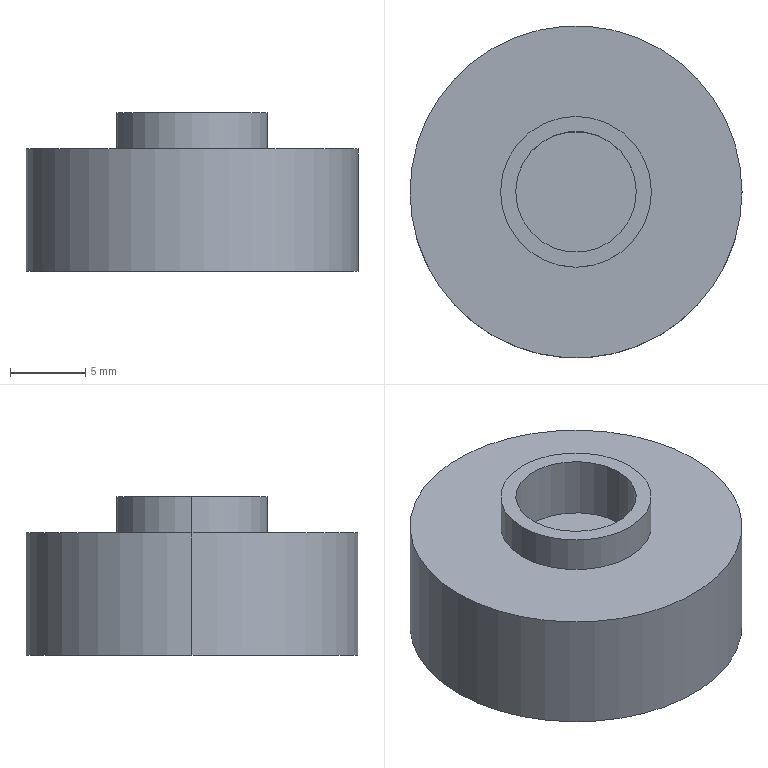Part | SolidWorks | features ICE 3, Chamfer 1, Extrusion 1 | 1 solid | 15 faces | box 22 x 22 x 10.5 mm | volume 2336 mm3 | cylinder 8 | plane 5 | cone 2 | commonest cylinder face diameters 8 x2 10 x2 17.5 x2 22 x2
STEP:
#1=CARTESIAN_POINT('',(8.75,0.,0.2));
#2=VERTEX_POINT('',#1);
#3=CARTESIAN_POINT('',(-8.75,0.,0.2));
#4=VERTEX_POINT('',#3);
#5=CARTESIAN_POINT('',(0.,0.,0.2));
#6=DIRECTION('',(0.,0.,-1.));
#7=DIRECTION('',(1.,0.,0.));
#8=AXIS2_PLACEMENT_3D('',#5,#6,#7);
#9=CIRCLE('',#8,8.75);
#10=EDGE_CURVE('',#2,#4,#9,.T.);
#11=ORIENTED_EDGE('',*,*,#10,.F.);
#12=CARTESIAN_POINT('',(8.95,0.,0.));
#13=VERTEX_POINT('',#12);
#14=CARTESIAN_POINT('',(8.75,0.,0.2));
#15=DIRECTION('',(0.7071,0.,-0.7071));
#16=VECTOR('',#15,1000.);
#17=LINE('',#14,#16);
#18=EDGE_CURVE('',#2,#13,#17,.T.);
#19=ORIENTED_EDGE('',*,*,#18,.T.);
#20=CARTESIAN_POINT('',(-8.95,0.,0.));
#21=VERTEX_POINT('',#20);
#22=CARTESIAN_POINT('',(0.,0.,0.));
#23=DIRECTION('',(0.,0.,1.));
#24=DIRECTION('',(1.,0.,0.));
#25=AXIS2_PLACEMENT_3D('',#22,#23,#24);
#26=CIRCLE('',#25,8.95);
#27=EDGE_CURVE('',#21,#13,#26,.T.);
#28=ORIENTED_EDGE('',*,*,#27,.F.);
#29=CARTESIAN_POINT('',(-8.75,0.,0.2));
#30=DIRECTION('',(-0.7071,0.,-0.7071));
#31=VECTOR('',#30,1000.);
#32=LINE('',#29,#31);
#33=EDGE_CURVE('',#4,#21,#32,.T.);
#34=ORIENTED_EDGE('',*,*,#33,.F.);
#35=EDGE_LOOP('',(#11,#19,#28,#34));
#36=FACE_OUTER_BOUND('',#35,.T.);
#37=CARTESIAN_POINT('',(0.,0.,0.2));
#38=DIRECTION('',(0.,0.,-1.));
#39=DIRECTION('',(-1.,0.,0.));
#40=AXIS2_PLACEMENT_3D('',#37,#38,#39);
#41=CONICAL_SURFACE('',#40,8.75,0.7854);
#42=ADVANCED_FACE('',(#36),#41,.F.);
#43=CARTESIAN_POINT('',(8.75,0.,3.));
#44=VERTEX_POINT('',#43);
#45=CARTESIAN_POINT('',(-8.75,0.,3.));
#46=VERTEX_POINT('',#45);
#47=CARTESIAN_POINT('',(0.,0.,3.));
#48=DIRECTION('',(0.,0.,-1.));
#49=DIRECTION('',(-1.,0.,0.));
#50=AXIS2_PLACEMENT_3D('',#47,#48,#49);
#51=CIRCLE('',#50,8.75);
#52=EDGE_CURVE('',#44,#46,#51,.T.);
#53=ORIENTED_EDGE('',*,*,#52,.F.);
#54=CARTESIAN_POINT('',(8.75,0.,3.));
#55=DIRECTION('',(0.,0.,-1.));
#56=VECTOR('',#55,1000.);
#57=LINE('',#54,#56);
#58=EDGE_CURVE('',#44,#2,#57,.T.);
#59=ORIENTED_EDGE('',*,*,#58,.T.);
#60=ORIENTED_EDGE('',*,*,#10,.T.);
#61=CARTESIAN_POINT('',(-8.75,0.,3.));
#62=DIRECTION('',(0.,0.,-1.));
#63=VECTOR('',#62,1000.);
#64=LINE('',#61,#63);
#65=EDGE_CURVE('',#46,#4,#64,.T.);
#66=ORIENTED_EDGE('',*,*,#65,.F.);
#67=EDGE_LOOP('',(#53,#59,#60,#66));
#68=FACE_OUTER_BOUND('',#67,.T.);
#69=CARTESIAN_POINT('',(0.,0.,3.));
#70=DIRECTION('',(0.,0.,-1.));
#71=DIRECTION('',(-1.,0.,0.));
#72=AXIS2_PLACEMENT_3D('',#69,#70,#71);
#73=CYLINDRICAL_SURFACE('',#72,8.75);
#74=ADVANCED_FACE('',(#68),#73,.F.);
#75=CARTESIAN_POINT('',(-4.,0.,6.35));
#76=VERTEX_POINT('',#75);
#77=CARTESIAN_POINT('',(4.,0.,6.35));
#78=VERTEX_POINT('',#77);
#79=CARTESIAN_POINT('',(0.,0.,6.35));
#80=DIRECTION('',(0.,0.,1.));
#81=DIRECTION('',(1.,0.,0.));
#82=AXIS2_PLACEMENT_3D('',#79,#80,#81);
#83=CIRCLE('',#82,4.);
#84=EDGE_CURVE('',#76,#78,#83,.T.);
#85=ORIENTED_EDGE('',*,*,#84,.F.);
#86=CARTESIAN_POINT('',(-4.,0.,10.5));
#87=VERTEX_POINT('',#86);
#88=CARTESIAN_POINT('',(-4.,0.,6.35));
#89=DIRECTION('',(0.,0.,1.));
#90=VECTOR('',#89,1000.);
#91=LINE('',#88,#90);
#92=EDGE_CURVE('',#76,#87,#91,.T.);
#93=ORIENTED_EDGE('',*,*,#92,.T.);
#94=CARTESIAN_POINT('',(4.,0.,10.5));
#95=VERTEX_POINT('',#94);
#96=CARTESIAN_POINT('',(0.,0.,10.5));
#97=DIRECTION('',(0.,0.,1.));
#98=DIRECTION('',(1.,0.,0.));
#99=AXIS2_PLACEMENT_3D('',#96,#97,#98);
#100=CIRCLE('',#99,4.);
#101=EDGE_CURVE('',#87,#95,#100,.T.);
#102=ORIENTED_EDGE('',*,*,#101,.T.);
#103=CARTESIAN_POINT('',(4.,0.,6.35));
#104=DIRECTION('',(0.,0.,1.));
#105=VECTOR('',#104,1000.);
#106=LINE('',#103,#105);
#107=EDGE_CURVE('',#78,#95,#106,.T.);
#108=ORIENTED_EDGE('',*,*,#107,.F.);
#109=EDGE_LOOP('',(#85,#93,#102,#108));
#110=FACE_OUTER_BOUND('',#109,.T.);
#111=CARTESIAN_POINT('',(0.,0.,6.35));
#112=DIRECTION('',(0.,0.,1.));
#113=DIRECTION('',(1.,0.,0.));
#114=AXIS2_PLACEMENT_3D('',#111,#112,#113);
#115=CYLINDRICAL_SURFACE('',#114,4.);
#116=ADVANCED_FACE('',(#110),#115,.F.);
#117=CARTESIAN_POINT('',(5.,0.,8.1));
#118=VERTEX_POINT('',#117);
#119=CARTESIAN_POINT('',(-5.,0.,8.1));
#120=VERTEX_POINT('',#119);
#121=CARTESIAN_POINT('',(0.,0.,8.1));
#122=DIRECTION('',(0.,0.,1.));
#123=DIRECTION('',(1.,0.,0.));
#124=AXIS2_PLACEMENT_3D('',#121,#122,#123);
#125=CIRCLE('',#124,5.);
#126=EDGE_CURVE('',#118,#120,#125,.T.);
#127=ORIENTED_EDGE('',*,*,#126,.T.);
#128=CARTESIAN_POINT('',(-5.,0.,10.5));
#129=VERTEX_POINT('',#128);
#130=CARTESIAN_POINT('',(-5.,0.,8.1));
#131=DIRECTION('',(0.,0.,1.));
#132=VECTOR('',#131,1000.);
#133=LINE('',#130,#132);
#134=EDGE_CURVE('',#120,#129,#133,.T.);
#135=ORIENTED_EDGE('',*,*,#134,.T.);
#136=CARTESIAN_POINT('',(5.,0.,10.5));
#137=VERTEX_POINT('',#136);
#138=CARTESIAN_POINT('',(0.,0.,10.5));
#139=DIRECTION('',(0.,0.,1.));
#140=DIRECTION('',(1.,0.,0.));
#141=AXIS2_PLACEMENT_3D('',#138,#139,#140);
#142=CIRCLE('',#141,5.);
#143=EDGE_CURVE('',#137,#129,#142,.T.);
#144=ORIENTED_EDGE('',*,*,#143,.F.);
#145=CARTESIAN_POINT('',(5.,0.,8.1));
#146=DIRECTION('',(0.,0.,1.));
#147=VECTOR('',#146,1000.);
#148=LINE('',#145,#147);
#149=EDGE_CURVE('',#118,#137,#148,.T.);
#150=ORIENTED_EDGE('',*,*,#149,.F.);
#151=EDGE_LOOP('',(#127,#135,#144,#150));
#152=FACE_OUTER_BOUND('',#151,.T.);
#153=CARTESIAN_POINT('',(0.,0.,8.1));
#154=DIRECTION('',(0.,0.,1.));
#155=DIRECTION('',(1.,0.,0.));
#156=AXIS2_PLACEMENT_3D('',#153,#154,#155);
#157=CYLINDRICAL_SURFACE('',#156,5.);
#158=ADVANCED_FACE('',(#152),#157,.T.);
#159=CARTESIAN_POINT('',(11.,0.,8.1));
#160=VERTEX_POINT('',#159);
#161=CARTESIAN_POINT('',(-11.,0.,8.1));
#162=VERTEX_POINT('',#161);
#163=CARTESIAN_POINT('',(0.,0.,8.1));
#164=DIRECTION('',(0.,0.,1.));
#165=DIRECTION('',(1.,0.,0.));
#166=AXIS2_PLACEMENT_3D('',#163,#164,#165);
#167=CIRCLE('',#166,11.);
#168=EDGE_CURVE('',#160,#162,#167,.T.);
#169=ORIENTED_EDGE('',*,*,#168,.F.);
#170=CARTESIAN_POINT('',(11.,0.,0.));
#171=VERTEX_POINT('',#170);
#172=CARTESIAN_POINT('',(11.,0.,10.5));
#173=DIRECTION('',(0.,0.,-1.));
#174=VECTOR('',#173,1000.);
#175=LINE('',#172,#174);
#176=EDGE_CURVE('',#160,#171,#175,.T.);
#177=ORIENTED_EDGE('',*,*,#176,.T.);
#178=CARTESIAN_POINT('',(-11.,0.,0.));
#179=VERTEX_POINT('',#178);
#180=CARTESIAN_POINT('',(0.,0.,0.));
#181=DIRECTION('',(0.,0.,1.));
#182=DIRECTION('',(1.,0.,0.));
#183=AXIS2_PLACEMENT_3D('',#180,#181,#182);
#184=CIRCLE('',#183,11.);
#185=EDGE_CURVE('',#171,#179,#184,.T.);
#186=ORIENTED_EDGE('',*,*,#185,.T.);
#187=CARTESIAN_POINT('',(-11.,0.,10.5));
#188=DIRECTION('',(0.,0.,-1.));
#189=VECTOR('',#188,1000.);
#190=LINE('',#187,#189);
#191=EDGE_CURVE('',#162,#179,#190,.T.);
#192=ORIENTED_EDGE('',*,*,#191,.F.);
#193=EDGE_LOOP('',(#169,#177,#186,#192));
#194=FACE_OUTER_BOUND('',#193,.T.);
#195=CARTESIAN_POINT('',(0.,0.,10.5));
#196=DIRECTION('',(0.,0.,-1.));
#197=DIRECTION('',(-1.,0.,0.));
#198=AXIS2_PLACEMENT_3D('',#195,#196,#197);
#199=CYLINDRICAL_SURFACE('',#198,11.);
#200=ADVANCED_FACE('',(#194),#199,.T.);
#201=ORIENTED_EDGE('',*,*,#176,.F.);
#202=CARTESIAN_POINT('',(0.,0.,8.1));
#203=DIRECTION('',(0.,0.,1.));
#204=DIRECTION('',(1.,0.,0.));
#205=AXIS2_PLACEMENT_3D('',#202,#203,#204);
#206=CIRCLE('',#205,11.);
#207=EDGE_CURVE('',#162,#160,#206,.T.);
#208=ORIENTED_EDGE('',*,*,#207,.F.);
#209=ORIENTED_EDGE('',*,*,#191,.T.);
#210=CARTESIAN_POINT('',(0.,0.,0.));
#211=DIRECTION('',(0.,0.,1.));
#212=DIRECTION('',(1.,0.,0.));
#213=AXIS2_PLACEMENT_3D('',#210,#211,#212);
#214=CIRCLE('',#213,11.);
#215=EDGE_CURVE('',#179,#171,#214,.T.);
#216=ORIENTED_EDGE('',*,*,#215,.T.);
#217=EDGE_LOOP('',(#201,#208,#209,#216));
#218=FACE_OUTER_BOUND('',#217,.T.);
#219=CARTESIAN_POINT('',(0.,0.,10.5));
#220=DIRECTION('',(0.,0.,-1.));
#221=DIRECTION('',(-1.,0.,0.));
#222=AXIS2_PLACEMENT_3D('',#219,#220,#221);
#223=CYLINDRICAL_SURFACE('',#222,11.);
#224=ADVANCED_FACE('',(#218),#223,.T.);
#225=ORIENTED_EDGE('',*,*,#27,.T.);
#226=CARTESIAN_POINT('',(0.,0.,0.));
#227=DIRECTION('',(0.,0.,1.));
#228=DIRECTION('',(1.,0.,0.));
#229=AXIS2_PLACEMENT_3D('',#226,#227,#228);
#230=CIRCLE('',#229,8.95);
#231=EDGE_CURVE('',#13,#21,#230,.T.);
#232=ORIENTED_EDGE('',*,*,#231,.T.);
#233=EDGE_LOOP('',(#225,#232));
#234=FACE_BOUND('',#233,.T.);
#235=ORIENTED_EDGE('',*,*,#215,.F.);
#236=ORIENTED_EDGE('',*,*,#185,.F.);
#237=EDGE_LOOP('',(#235,#236));
#238=FACE_OUTER_BOUND('',#237,.T.);
#239=CARTESIAN_POINT('',(0.,0.,0.));
#240=DIRECTION('',(0.,0.,1.));
#241=DIRECTION('',(1.,0.,0.));
#242=AXIS2_PLACEMENT_3D('',#239,#240,#241);
#243=PLANE('',#242);
#244=ADVANCED_FACE('',(#234,#238),#243,.F.);
#245=ORIENTED_EDGE('',*,*,#126,.F.);
#246=CARTESIAN_POINT('',(0.,0.,8.1));
#247=DIRECTION('',(0.,0.,1.));
#248=DIRECTION('',(1.,0.,0.));
#249=AXIS2_PLACEMENT_3D('',#246,#247,#248);
#250=CIRCLE('',#249,5.);
#251=EDGE_CURVE('',#120,#118,#250,.T.);
#252=ORIENTED_EDGE('',*,*,#251,.F.);
#253=EDGE_LOOP('',(#245,#252));
#254=FACE_BOUND('',#253,.T.);
#255=ORIENTED_EDGE('',*,*,#207,.T.);
#256=ORIENTED_EDGE('',*,*,#168,.T.);
#257=EDGE_LOOP('',(#255,#256));
#258=FACE_OUTER_BOUND('',#257,.T.);
#259=CARTESIAN_POINT('',(0.,0.,8.1));
#260=DIRECTION('',(0.,0.,1.));
#261=DIRECTION('',(1.,0.,0.));
#262=AXIS2_PLACEMENT_3D('',#259,#260,#261);
#263=PLANE('',#262);
#264=ADVANCED_FACE('',(#254,#258),#263,.T.);
#265=ORIENTED_EDGE('',*,*,#134,.F.);
#266=ORIENTED_EDGE('',*,*,#251,.T.);
#267=ORIENTED_EDGE('',*,*,#149,.T.);
#268=CARTESIAN_POINT('',(0.,0.,10.5));
#269=DIRECTION('',(0.,0.,1.));
#270=DIRECTION('',(1.,0.,0.));
#271=AXIS2_PLACEMENT_3D('',#268,#269,#270);
#272=CIRCLE('',#271,5.);
#273=EDGE_CURVE('',#129,#137,#272,.T.);
#274=ORIENTED_EDGE('',*,*,#273,.F.);
#275=EDGE_LOOP('',(#265,#266,#267,#274));
#276=FACE_OUTER_BOUND('',#275,.T.);
#277=CARTESIAN_POINT('',(0.,0.,8.1));
#278=DIRECTION('',(0.,0.,1.));
#279=DIRECTION('',(1.,0.,0.));
#280=AXIS2_PLACEMENT_3D('',#277,#278,#279);
#281=CYLINDRICAL_SURFACE('',#280,5.);
#282=ADVANCED_FACE('',(#276),#281,.T.);
#283=CARTESIAN_POINT('',(0.,0.,10.5));
#284=DIRECTION('',(0.,0.,1.));
#285=DIRECTION('',(1.,0.,0.));
#286=AXIS2_PLACEMENT_3D('',#283,#284,#285);
#287=CIRCLE('',#286,4.);
#288=EDGE_CURVE('',#95,#87,#287,.T.);
#289=ORIENTED_EDGE('',*,*,#288,.F.);
#290=ORIENTED_EDGE('',*,*,#101,.F.);
#291=EDGE_LOOP('',(#289,#290));
#292=FACE_BOUND('',#291,.T.);
#293=ORIENTED_EDGE('',*,*,#143,.T.);
#294=ORIENTED_EDGE('',*,*,#273,.T.);
#295=EDGE_LOOP('',(#293,#294));
#296=FACE_OUTER_BOUND('',#295,.T.);
#297=CARTESIAN_POINT('',(0.,0.,10.5));
#298=DIRECTION('',(0.,0.,1.));
#299=DIRECTION('',(1.,0.,0.));
#300=AXIS2_PLACEMENT_3D('',#297,#298,#299);
#301=PLANE('',#300);
#302=ADVANCED_FACE('',(#292,#296),#301,.T.);
#303=ORIENTED_EDGE('',*,*,#92,.F.);
#304=CARTESIAN_POINT('',(0.,0.,6.35));
#305=DIRECTION('',(0.,0.,1.));
#306=DIRECTION('',(1.,0.,0.));
#307=AXIS2_PLACEMENT_3D('',#304,#305,#306);
#308=CIRCLE('',#307,4.);
#309=EDGE_CURVE('',#78,#76,#308,.T.);
#310=ORIENTED_EDGE('',*,*,#309,.F.);
#311=ORIENTED_EDGE('',*,*,#107,.T.);
#312=ORIENTED_EDGE('',*,*,#288,.T.);
#313=EDGE_LOOP('',(#303,#310,#311,#312));
#314=FACE_OUTER_BOUND('',#313,.T.);
#315=CARTESIAN_POINT('',(0.,0.,6.35));
#316=DIRECTION('',(0.,0.,1.));
#317=DIRECTION('',(1.,0.,0.));
#318=AXIS2_PLACEMENT_3D('',#315,#316,#317);
#319=CYLINDRICAL_SURFACE('',#318,4.);
#320=ADVANCED_FACE('',(#314),#319,.F.);
#321=ORIENTED_EDGE('',*,*,#309,.T.);
#322=ORIENTED_EDGE('',*,*,#84,.T.);
#323=EDGE_LOOP('',(#321,#322));
#324=FACE_OUTER_BOUND('',#323,.T.);
#325=CARTESIAN_POINT('',(0.,0.,6.35));
#326=DIRECTION('',(0.,0.,1.));
#327=DIRECTION('',(1.,0.,0.));
#328=AXIS2_PLACEMENT_3D('',#325,#326,#327);
#329=PLANE('',#328);
#330=ADVANCED_FACE('',(#324),#329,.T.);
#331=ORIENTED_EDGE('',*,*,#58,.F.);
#332=CARTESIAN_POINT('',(0.,0.,3.));
#333=DIRECTION('',(0.,0.,-1.));
#334=DIRECTION('',(-1.,0.,0.));
#335=AXIS2_PLACEMENT_3D('',#332,#333,#334);
#336=CIRCLE('',#335,8.75);
#337=EDGE_CURVE('',#46,#44,#336,.T.);
#338=ORIENTED_EDGE('',*,*,#337,.F.);
#339=ORIENTED_EDGE('',*,*,#65,.T.);
#340=CARTESIAN_POINT('',(0.,0.,0.2));
#341=DIRECTION('',(0.,0.,-1.));
#342=DIRECTION('',(1.,0.,0.));
#343=AXIS2_PLACEMENT_3D('',#340,#341,#342);
#344=CIRCLE('',#343,8.75);
#345=EDGE_CURVE('',#4,#2,#344,.T.);
#346=ORIENTED_EDGE('',*,*,#345,.T.);
#347=EDGE_LOOP('',(#331,#338,#339,#346));
#348=FACE_OUTER_BOUND('',#347,.T.);
#349=CARTESIAN_POINT('',(0.,0.,3.));
#350=DIRECTION('',(0.,0.,-1.));
#351=DIRECTION('',(-1.,0.,0.));
#352=AXIS2_PLACEMENT_3D('',#349,#350,#351);
#353=CYLINDRICAL_SURFACE('',#352,8.75);
#354=ADVANCED_FACE('',(#348),#353,.F.);
#355=ORIENTED_EDGE('',*,*,#337,.T.);
#356=ORIENTED_EDGE('',*,*,#52,.T.);
#357=EDGE_LOOP('',(#355,#356));
#358=FACE_OUTER_BOUND('',#357,.T.);
#359=CARTESIAN_POINT('',(0.,0.,3.));
#360=DIRECTION('',(0.,0.,-1.));
#361=DIRECTION('',(-1.,0.,0.));
#362=AXIS2_PLACEMENT_3D('',#359,#360,#361);
#363=PLANE('',#362);
#364=ADVANCED_FACE('',(#358),#363,.T.);
#365=ORIENTED_EDGE('',*,*,#18,.F.);
#366=ORIENTED_EDGE('',*,*,#345,.F.);
#367=ORIENTED_EDGE('',*,*,#33,.T.);
#368=ORIENTED_EDGE('',*,*,#231,.F.);
#369=EDGE_LOOP('',(#365,#366,#367,#368));
#370=FACE_OUTER_BOUND('',#369,.T.);
#371=CARTESIAN_POINT('',(0.,0.,0.2));
#372=DIRECTION('',(0.,0.,-1.));
#373=DIRECTION('',(-1.,0.,0.));
#374=AXIS2_PLACEMENT_3D('',#371,#372,#373);
#375=CONICAL_SURFACE('',#374,8.75,0.7854);
#376=ADVANCED_FACE('',(#370),#375,.F.);
#377=CLOSED_SHELL('',(#42,#74,#116,#158,#200,#224,#244,#264,#282,#302,#320,#330,#354,#364,#376));
#378=MANIFOLD_SOLID_BREP('',#377);
#379=CARTESIAN_POINT('',(0.,0.,0.));
#380=DIRECTION('',(0.,0.,1.));
#381=DIRECTION('',(1.,0.,0.));
#382=AXIS2_PLACEMENT_3D('',#379,#380,#381);
#383=(LENGTH_UNIT()NAMED_UNIT(*)SI_UNIT(.MILLI.,.METRE.));
#384=UNCERTAINTY_MEASURE_WITH_UNIT(LENGTH_MEASURE(0.00001),#383,'','');
#385=(NAMED_UNIT(*)PLANE_ANGLE_UNIT()SI_UNIT($,.RADIAN.));
#386=(NAMED_UNIT(*)SI_UNIT($,.STERADIAN.)SOLID_ANGLE_UNIT());
#387=(GEOMETRIC_REPRESENTATION_CONTEXT(3)GLOBAL_UNCERTAINTY_ASSIGNED_CONTEXT((#384))GLOBAL_UNIT_ASSIGNED_CONTEXT((#383,#385,#386))REPRESENTATION_CONTEXT('',''));
#388=ADVANCED_BREP_SHAPE_REPRESENTATION('',(#378,#382),#387);